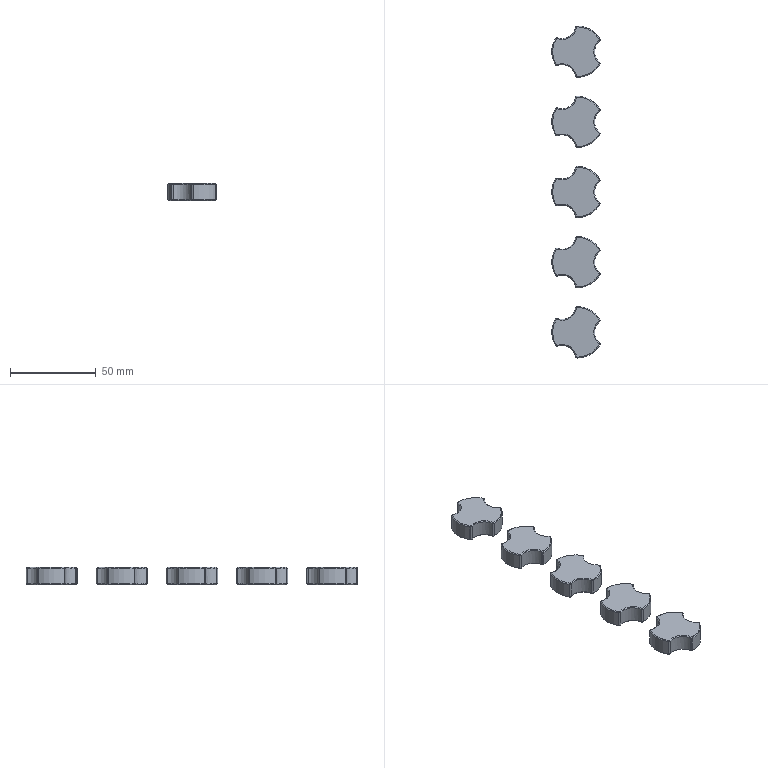NC program | NX | posted with a generic post | part box 28.194 x 194 x 10 mm
Lines 1 to 18 of 9608:
N10 G17 G21 G94 G90
(FLOOR_WALL , TOOL : D80)
N12 T19 M6
N14 G54
N16 G17 G0 G90 X-144. Y0. S6500 M3
N18 G43 Z30. H19
N20 Z3.
N22 G94 G1 Z0. F1500.
N24 X-139.
N26 X139.
N28 X144.
N30 Z3.
N32 G0 Z30.
N34 M5